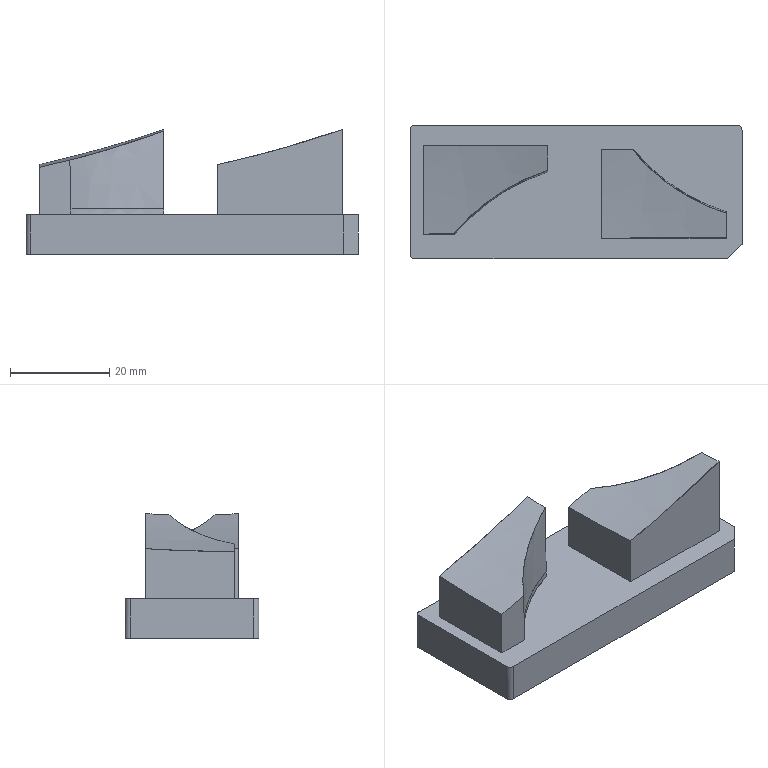CAM job | PowerMill | 3-axis milling, other | part box 67 x 27 x 25.167 mm
Tools:
number,name,type,diameter,tip_radius,length,cutting_length,overhang,flutes,holder,toolpaths_using
1,D10C,end_mill,10.0,0.0,60.0,,30.0,1,D42L35,1
1,D10C_1_1_1,end_mill,10.0,0.0,60.0,,25.6,1,D42L35,3
2,D4C_1_1,end_mill,4.0,0.0,30.0,,17.36,1,D42L35,2
3,D10_1_1_1,end_mill,10.0,0.0,60.0,,25.32,1,D42L35,3
7,R2_1_1,ball_nosed,4.0,2.0,30.0,,7.96,1,D42L35,1
14,D4_1_1,end_mill,4.0,0.0,30.0,,16.6,1,D42L35,1
13,Text_D4_1_1,taper_spherical,4.0,0.3,60.0,,17.44,1,D42L35,1
Operations:
program,toolpath,strategy,tool,tool_number,tool_diameter,tip_radius,flutes,spindle_rpm,feed_cut,surface_speed_m_min_computed,feed_per_tooth_computed,tolerance,thickness,stepover,stepdown,cut_length,cut_time_min,total_time_min,workplane
20-C01-14-F,精公开粗01-扫面平行-D10C,raster_area_clear,D10C_1_1_1,1,10.0,0.0,1.0,8000.0,10000.0,251.33,1.25,0.03,0.28,6.0,1.0,540.48,0.054,0.0616,
20-C01-14-F,精公开粗01-外形偏置-D10C,offset_area_clear,D10C_1_1_1,1,10.0,0.0,1.0,8000.0,10000.0,251.33,1.25,0.03,0.28,6.0,1.0,22623.961,2.262,2.37,
20-C01-14-F,精公开粗01-基准台等高-D10C,constantz,D10C_1_1_1,1,10.0,0.0,1.0,8000.0,10000.0,251.33,1.25,0.03,0.07,5.0,0.4,4769.075,0.477,0.4893,
20-C01-14-F,精公再粗02-外形偏置-D4C,offset_area_clear,D4C_1_1,2,4.0,0.0,1.0,18000.0,6000.0,226.19,0.3333,0.03,0.0,2.0,1.0,13586.492,2.264,2.343,
20-C01-14-F,精公再粗02-平行中光-D4C,raster,D4C_1_1,2,4.0,0.0,1.0,18000.0,6000.0,226.19,0.3333,0.03,0.0,0.2,1.0,4573.77,0.762,0.7896,
20-C01-14-F,精公基准台01-基准面偏置-D10,offset_area_clear,D10_1_1_1,3,10.0,0.0,1.0,8500.0,600.0,267.04,0.0706,0.005,0.38,5.0,1.0,319.538,0.532,0.5786,
20-C01-14-F,精公基准台01-外形侧光-D10,profile_area_clear,D10_1_1_1,3,10.0,0.0,1.0,8500.0,600.0,267.04,0.0706,0.005,-0.07,0.08,1.0,434.974,0.725,0.7722,
20-C01-14-F,精公基准台01-基准台侧光-D10,profile_area_clear,D10_1_1_1,3,10.0,0.0,1.0,8500.0,600.0,267.04,0.0706,0.005,0.0,0.08,1.0,433.233,0.722,0.7891,
20-C01-14-F,精公精光01-平行-R2,raster,R2_1_1,7,4.0,2.0,1.0,18000.0,2000.0,226.19,0.1111,0.005,-0.075,0.05,1.0,12559.672,6.28,6.333,
20-C01-14-F,精公精光02-等高-D4,constantz,D4_1_1,14,4.0,0.0,1.0,18000.0,2000.0,226.19,0.1111,0.005,-0.075,5.0,0.06,9514.871,4.757,5.247,
20-C01-14-F,精公刻字01-刻字-Text_D4,pattern,Text_D4_1_1,13,4.0,0.3,1.0,15000.0,1000.0,188.5,0.0667,0.005,0.0,5.0,1.0,55.163,0.055,0.0769,
,精公开粗01-外形偏置-D10C_Reference,offset_area_clear,D10C,1,10.0,0.0,1.0,8000.0,10000.0,251.33,1.25,0.03,0.28,6.0,1.0,45266.598,4.527,4.738,